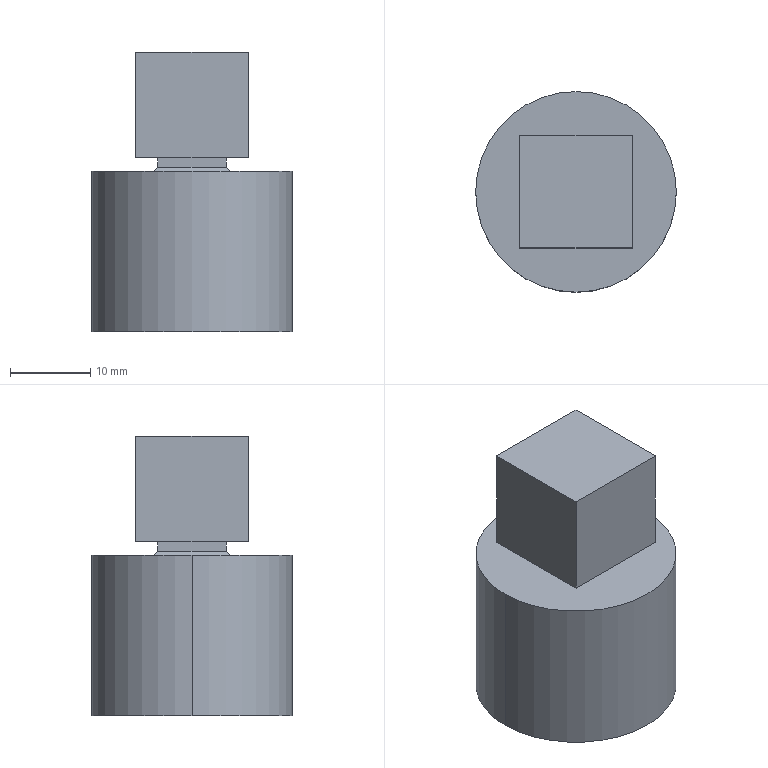Part | SolidWorks | features ICE 3, Chamfer 1, Extrusion 1 | 1 solid | 21 faces | box 25 x 25 x 34.87 mm | volume 7814 mm3 | plane 17 | cylinder 4 | commonest cylinder face diameters 20 x2 25 x2
STEP:
#1=CARTESIAN_POINT('',(10.,0.,15.));
#2=VERTEX_POINT('',#1);
#3=CARTESIAN_POINT('',(-10.,0.,15.));
#4=VERTEX_POINT('',#3);
#5=CARTESIAN_POINT('',(0.,0.,15.));
#6=DIRECTION('',(0.,0.,-1.));
#7=DIRECTION('',(-1.,0.,0.));
#8=AXIS2_PLACEMENT_3D('',#5,#6,#7);
#9=CIRCLE('',#8,10.);
#10=EDGE_CURVE('',#2,#4,#9,.T.);
#11=ORIENTED_EDGE('',*,*,#10,.F.);
#12=CARTESIAN_POINT('',(10.,0.,0.));
#13=VERTEX_POINT('',#12);
#14=CARTESIAN_POINT('',(10.,0.,15.));
#15=DIRECTION('',(0.,0.,-1.));
#16=VECTOR('',#15,1000.);
#17=LINE('',#14,#16);
#18=EDGE_CURVE('',#2,#13,#17,.T.);
#19=ORIENTED_EDGE('',*,*,#18,.T.);
#20=CARTESIAN_POINT('',(-10.,0.,0.));
#21=VERTEX_POINT('',#20);
#22=CARTESIAN_POINT('',(0.,0.,0.));
#23=DIRECTION('',(0.,0.,-1.));
#24=DIRECTION('',(-1.,0.,0.));
#25=AXIS2_PLACEMENT_3D('',#22,#23,#24);
#26=CIRCLE('',#25,10.);
#27=EDGE_CURVE('',#13,#21,#26,.T.);
#28=ORIENTED_EDGE('',*,*,#27,.T.);
#29=CARTESIAN_POINT('',(-10.,0.,15.));
#30=DIRECTION('',(0.,0.,-1.));
#31=VECTOR('',#30,1000.);
#32=LINE('',#29,#31);
#33=EDGE_CURVE('',#4,#21,#32,.T.);
#34=ORIENTED_EDGE('',*,*,#33,.F.);
#35=EDGE_LOOP('',(#11,#19,#28,#34));
#36=FACE_OUTER_BOUND('',#35,.T.);
#37=CARTESIAN_POINT('',(0.,0.,15.));
#38=DIRECTION('',(0.,0.,-1.));
#39=DIRECTION('',(-1.,0.,0.));
#40=AXIS2_PLACEMENT_3D('',#37,#38,#39);
#41=CYLINDRICAL_SURFACE('',#40,10.);
#42=ADVANCED_FACE('',(#36),#41,.F.);
#43=CARTESIAN_POINT('',(12.5,0.,20.));
#44=VERTEX_POINT('',#43);
#45=CARTESIAN_POINT('',(-12.5,0.,20.));
#46=VERTEX_POINT('',#45);
#47=CARTESIAN_POINT('',(0.,0.,20.));
#48=DIRECTION('',(0.,0.,1.));
#49=DIRECTION('',(1.,0.,0.));
#50=AXIS2_PLACEMENT_3D('',#47,#48,#49);
#51=CIRCLE('',#50,12.5);
#52=EDGE_CURVE('',#44,#46,#51,.T.);
#53=ORIENTED_EDGE('',*,*,#52,.F.);
#54=CARTESIAN_POINT('',(12.5,0.,0.));
#55=VERTEX_POINT('',#54);
#56=CARTESIAN_POINT('',(12.5,0.,20.));
#57=DIRECTION('',(0.,0.,-1.));
#58=VECTOR('',#57,1000.);
#59=LINE('',#56,#58);
#60=EDGE_CURVE('',#44,#55,#59,.T.);
#61=ORIENTED_EDGE('',*,*,#60,.T.);
#62=CARTESIAN_POINT('',(-12.5,0.,0.));
#63=VERTEX_POINT('',#62);
#64=CARTESIAN_POINT('',(0.,0.,0.));
#65=DIRECTION('',(0.,0.,1.));
#66=DIRECTION('',(1.,0.,0.));
#67=AXIS2_PLACEMENT_3D('',#64,#65,#66);
#68=CIRCLE('',#67,12.5);
#69=EDGE_CURVE('',#55,#63,#68,.T.);
#70=ORIENTED_EDGE('',*,*,#69,.T.);
#71=CARTESIAN_POINT('',(-12.5,0.,20.));
#72=DIRECTION('',(0.,0.,-1.));
#73=VECTOR('',#72,1000.);
#74=LINE('',#71,#73);
#75=EDGE_CURVE('',#46,#63,#74,.T.);
#76=ORIENTED_EDGE('',*,*,#75,.F.);
#77=EDGE_LOOP('',(#53,#61,#70,#76));
#78=FACE_OUTER_BOUND('',#77,.T.);
#79=CARTESIAN_POINT('',(0.,0.,20.));
#80=DIRECTION('',(0.,0.,-1.));
#81=DIRECTION('',(-1.,0.,0.));
#82=AXIS2_PLACEMENT_3D('',#79,#80,#81);
#83=CYLINDRICAL_SURFACE('',#82,12.5);
#84=ADVANCED_FACE('',(#78),#83,.T.);
#85=ORIENTED_EDGE('',*,*,#60,.F.);
#86=CARTESIAN_POINT('',(0.,0.,20.));
#87=DIRECTION('',(0.,0.,1.));
#88=DIRECTION('',(1.,0.,0.));
#89=AXIS2_PLACEMENT_3D('',#86,#87,#88);
#90=CIRCLE('',#89,12.5);
#91=EDGE_CURVE('',#46,#44,#90,.T.);
#92=ORIENTED_EDGE('',*,*,#91,.F.);
#93=ORIENTED_EDGE('',*,*,#75,.T.);
#94=CARTESIAN_POINT('',(0.,0.,0.));
#95=DIRECTION('',(0.,0.,1.));
#96=DIRECTION('',(1.,0.,0.));
#97=AXIS2_PLACEMENT_3D('',#94,#95,#96);
#98=CIRCLE('',#97,12.5);
#99=EDGE_CURVE('',#63,#55,#98,.T.);
#100=ORIENTED_EDGE('',*,*,#99,.T.);
#101=EDGE_LOOP('',(#85,#92,#93,#100));
#102=FACE_OUTER_BOUND('',#101,.T.);
#103=CARTESIAN_POINT('',(0.,0.,20.));
#104=DIRECTION('',(0.,0.,-1.));
#105=DIRECTION('',(-1.,0.,0.));
#106=AXIS2_PLACEMENT_3D('',#103,#104,#105);
#107=CYLINDRICAL_SURFACE('',#106,12.5);
#108=ADVANCED_FACE('',(#102),#107,.T.);
#109=CARTESIAN_POINT('',(4.75,4.75,20.));
#110=VERTEX_POINT('',#109);
#111=CARTESIAN_POINT('',(4.75,-4.75,20.));
#112=VERTEX_POINT('',#111);
#113=CARTESIAN_POINT('',(4.75,0.,20.));
#114=DIRECTION('',(0.,-1.,0.));
#115=VECTOR('',#114,1000.);
#116=LINE('',#113,#115);
#117=EDGE_CURVE('',#110,#112,#116,.T.);
#118=ORIENTED_EDGE('',*,*,#117,.T.);
#119=CARTESIAN_POINT('',(-4.75,-4.75,20.));
#120=VERTEX_POINT('',#119);
#121=CARTESIAN_POINT('',(0.,-4.75,20.));
#122=DIRECTION('',(-1.,0.,0.));
#123=VECTOR('',#122,1000.);
#124=LINE('',#121,#123);
#125=EDGE_CURVE('',#112,#120,#124,.T.);
#126=ORIENTED_EDGE('',*,*,#125,.T.);
#127=CARTESIAN_POINT('',(-4.75,4.75,20.));
#128=VERTEX_POINT('',#127);
#129=CARTESIAN_POINT('',(-4.75,0.,20.));
#130=DIRECTION('',(0.,1.,0.));
#131=VECTOR('',#130,1000.);
#132=LINE('',#129,#131);
#133=EDGE_CURVE('',#120,#128,#132,.T.);
#134=ORIENTED_EDGE('',*,*,#133,.T.);
#135=CARTESIAN_POINT('',(0.,4.75,20.));
#136=DIRECTION('',(1.,0.,0.));
#137=VECTOR('',#136,1000.);
#138=LINE('',#135,#137);
#139=EDGE_CURVE('',#128,#110,#138,.T.);
#140=ORIENTED_EDGE('',*,*,#139,.T.);
#141=EDGE_LOOP('',(#118,#126,#134,#140));
#142=FACE_BOUND('',#141,.T.);
#143=ORIENTED_EDGE('',*,*,#91,.T.);
#144=ORIENTED_EDGE('',*,*,#52,.T.);
#145=EDGE_LOOP('',(#143,#144));
#146=FACE_OUTER_BOUND('',#145,.T.);
#147=CARTESIAN_POINT('',(0.,0.,20.));
#148=DIRECTION('',(0.,0.,1.));
#149=DIRECTION('',(1.,0.,0.));
#150=AXIS2_PLACEMENT_3D('',#147,#148,#149);
#151=PLANE('',#150);
#152=ADVANCED_FACE('',(#142,#146),#151,.T.);
#153=CARTESIAN_POINT('',(0.,0.,0.));
#154=DIRECTION('',(0.,0.,-1.));
#155=DIRECTION('',(-1.,0.,0.));
#156=AXIS2_PLACEMENT_3D('',#153,#154,#155);
#157=CIRCLE('',#156,10.);
#158=EDGE_CURVE('',#21,#13,#157,.T.);
#159=ORIENTED_EDGE('',*,*,#158,.F.);
#160=ORIENTED_EDGE('',*,*,#27,.F.);
#161=EDGE_LOOP('',(#159,#160));
#162=FACE_BOUND('',#161,.T.);
#163=ORIENTED_EDGE('',*,*,#99,.F.);
#164=ORIENTED_EDGE('',*,*,#69,.F.);
#165=EDGE_LOOP('',(#163,#164));
#166=FACE_OUTER_BOUND('',#165,.T.);
#167=CARTESIAN_POINT('',(0.,0.,0.));
#168=DIRECTION('',(0.,0.,1.));
#169=DIRECTION('',(1.,0.,0.));
#170=AXIS2_PLACEMENT_3D('',#167,#168,#169);
#171=PLANE('',#170);
#172=ADVANCED_FACE('',(#162,#166),#171,.F.);
#173=CARTESIAN_POINT('',(4.25,-4.25,21.7));
#174=VERTEX_POINT('',#173);
#175=CARTESIAN_POINT('',(4.25,-4.25,20.5));
#176=VERTEX_POINT('',#175);
#177=CARTESIAN_POINT('',(4.25,-4.25,21.7));
#178=DIRECTION('',(0.,0.,-1.));
#179=VECTOR('',#178,1000.);
#180=LINE('',#177,#179);
#181=EDGE_CURVE('',#174,#176,#180,.T.);
#182=ORIENTED_EDGE('',*,*,#181,.T.);
#183=CARTESIAN_POINT('',(4.25,4.25,20.5));
#184=VERTEX_POINT('',#183);
#185=CARTESIAN_POINT('',(4.25,-4.25,20.5));
#186=DIRECTION('',(0.,1.,0.));
#187=VECTOR('',#186,1000.);
#188=LINE('',#185,#187);
#189=EDGE_CURVE('',#176,#184,#188,.T.);
#190=ORIENTED_EDGE('',*,*,#189,.T.);
#191=CARTESIAN_POINT('',(4.25,4.25,21.7));
#192=VERTEX_POINT('',#191);
#193=CARTESIAN_POINT('',(4.25,4.25,21.7));
#194=DIRECTION('',(0.,0.,-1.));
#195=VECTOR('',#194,1000.);
#196=LINE('',#193,#195);
#197=EDGE_CURVE('',#192,#184,#196,.T.);
#198=ORIENTED_EDGE('',*,*,#197,.F.);
#199=CARTESIAN_POINT('',(4.25,-4.25,21.7));
#200=DIRECTION('',(0.,1.,0.));
#201=VECTOR('',#200,1000.);
#202=LINE('',#199,#201);
#203=EDGE_CURVE('',#174,#192,#202,.T.);
#204=ORIENTED_EDGE('',*,*,#203,.F.);
#205=EDGE_LOOP('',(#182,#190,#198,#204));
#206=FACE_OUTER_BOUND('',#205,.T.);
#207=CARTESIAN_POINT('',(4.25,-4.25,21.7));
#208=DIRECTION('',(-1.,0.,0.));
#209=DIRECTION('',(0.,0.,1.));
#210=AXIS2_PLACEMENT_3D('',#207,#208,#209);
#211=PLANE('',#210);
#212=ADVANCED_FACE('',(#206),#211,.F.);
#213=ORIENTED_EDGE('',*,*,#197,.T.);
#214=CARTESIAN_POINT('',(-4.25,4.25,20.5));
#215=VERTEX_POINT('',#214);
#216=CARTESIAN_POINT('',(-4.25,4.25,20.5));
#217=DIRECTION('',(-1.,0.,0.));
#218=VECTOR('',#217,1000.);
#219=LINE('',#216,#218);
#220=EDGE_CURVE('',#184,#215,#219,.T.);
#221=ORIENTED_EDGE('',*,*,#220,.T.);
#222=CARTESIAN_POINT('',(-4.25,4.25,21.7));
#223=VERTEX_POINT('',#222);
#224=CARTESIAN_POINT('',(-4.25,4.25,21.7));
#225=DIRECTION('',(0.,0.,-1.));
#226=VECTOR('',#225,1000.);
#227=LINE('',#224,#226);
#228=EDGE_CURVE('',#223,#215,#227,.T.);
#229=ORIENTED_EDGE('',*,*,#228,.F.);
#230=CARTESIAN_POINT('',(-4.25,4.25,21.7));
#231=DIRECTION('',(-1.,0.,0.));
#232=VECTOR('',#231,1000.);
#233=LINE('',#230,#232);
#234=EDGE_CURVE('',#192,#223,#233,.T.);
#235=ORIENTED_EDGE('',*,*,#234,.F.);
#236=EDGE_LOOP('',(#213,#221,#229,#235));
#237=FACE_OUTER_BOUND('',#236,.T.);
#238=CARTESIAN_POINT('',(-4.25,4.25,21.7));
#239=DIRECTION('',(0.,-1.,0.));
#240=DIRECTION('',(0.,0.,-1.));
#241=AXIS2_PLACEMENT_3D('',#238,#239,#240);
#242=PLANE('',#241);
#243=ADVANCED_FACE('',(#237),#242,.F.);
#244=ORIENTED_EDGE('',*,*,#228,.T.);
#245=CARTESIAN_POINT('',(-4.25,-4.25,20.5));
#246=VERTEX_POINT('',#245);
#247=CARTESIAN_POINT('',(-4.25,-4.25,20.5));
#248=DIRECTION('',(0.,-1.,0.));
#249=VECTOR('',#248,1000.);
#250=LINE('',#247,#249);
#251=EDGE_CURVE('',#215,#246,#250,.T.);
#252=ORIENTED_EDGE('',*,*,#251,.T.);
#253=CARTESIAN_POINT('',(-4.25,-4.25,21.7));
#254=VERTEX_POINT('',#253);
#255=CARTESIAN_POINT('',(-4.25,-4.25,21.7));
#256=DIRECTION('',(0.,0.,-1.));
#257=VECTOR('',#256,1000.);
#258=LINE('',#255,#257);
#259=EDGE_CURVE('',#254,#246,#258,.T.);
#260=ORIENTED_EDGE('',*,*,#259,.F.);
#261=CARTESIAN_POINT('',(-4.25,-4.25,21.7));
#262=DIRECTION('',(0.,-1.,0.));
#263=VECTOR('',#262,1000.);
#264=LINE('',#261,#263);
#265=EDGE_CURVE('',#223,#254,#264,.T.);
#266=ORIENTED_EDGE('',*,*,#265,.F.);
#267=EDGE_LOOP('',(#244,#252,#260,#266));
#268=FACE_OUTER_BOUND('',#267,.T.);
#269=CARTESIAN_POINT('',(-4.25,-4.25,21.7));
#270=DIRECTION('',(1.,0.,0.));
#271=DIRECTION('',(0.,0.,-1.));
#272=AXIS2_PLACEMENT_3D('',#269,#270,#271);
#273=PLANE('',#272);
#274=ADVANCED_FACE('',(#268),#273,.F.);
#275=ORIENTED_EDGE('',*,*,#259,.T.);
#276=CARTESIAN_POINT('',(-4.25,-4.25,20.5));
#277=DIRECTION('',(1.,0.,0.));
#278=VECTOR('',#277,1000.);
#279=LINE('',#276,#278);
#280=EDGE_CURVE('',#246,#176,#279,.T.);
#281=ORIENTED_EDGE('',*,*,#280,.T.);
#282=ORIENTED_EDGE('',*,*,#181,.F.);
#283=CARTESIAN_POINT('',(-4.25,-4.25,21.7));
#284=DIRECTION('',(1.,0.,0.));
#285=VECTOR('',#284,1000.);
#286=LINE('',#283,#285);
#287=EDGE_CURVE('',#254,#174,#286,.T.);
#288=ORIENTED_EDGE('',*,*,#287,.F.);
#289=EDGE_LOOP('',(#275,#281,#282,#288));
#290=FACE_OUTER_BOUND('',#289,.T.);
#291=CARTESIAN_POINT('',(-4.25,-4.25,21.7));
#292=DIRECTION('',(0.,1.,0.));
#293=DIRECTION('',(0.,0.,1.));
#294=AXIS2_PLACEMENT_3D('',#291,#292,#293);
#295=PLANE('',#294);
#296=ADVANCED_FACE('',(#290),#295,.F.);
#297=CARTESIAN_POINT('',(7.,-7.,21.7));
#298=VERTEX_POINT('',#297);
#299=CARTESIAN_POINT('',(7.,7.,21.7));
#300=VERTEX_POINT('',#299);
#301=CARTESIAN_POINT('',(7.,-7.,21.7));
#302=DIRECTION('',(0.,1.,0.));
#303=VECTOR('',#302,1000.);
#304=LINE('',#301,#303);
#305=EDGE_CURVE('',#298,#300,#304,.T.);
#306=ORIENTED_EDGE('',*,*,#305,.T.);
#307=CARTESIAN_POINT('',(7.,7.,34.87));
#308=VERTEX_POINT('',#307);
#309=CARTESIAN_POINT('',(7.,7.,34.87));
#310=DIRECTION('',(0.,0.,-1.));
#311=VECTOR('',#310,1000.);
#312=LINE('',#309,#311);
#313=EDGE_CURVE('',#308,#300,#312,.T.);
#314=ORIENTED_EDGE('',*,*,#313,.F.);
#315=CARTESIAN_POINT('',(7.,-7.,34.87));
#316=VERTEX_POINT('',#315);
#317=CARTESIAN_POINT('',(7.,-7.,34.87));
#318=DIRECTION('',(0.,1.,0.));
#319=VECTOR('',#318,1000.);
#320=LINE('',#317,#319);
#321=EDGE_CURVE('',#316,#308,#320,.T.);
#322=ORIENTED_EDGE('',*,*,#321,.F.);
#323=CARTESIAN_POINT('',(7.,-7.,34.87));
#324=DIRECTION('',(0.,0.,-1.));
#325=VECTOR('',#324,1000.);
#326=LINE('',#323,#325);
#327=EDGE_CURVE('',#316,#298,#326,.T.);
#328=ORIENTED_EDGE('',*,*,#327,.T.);
#329=EDGE_LOOP('',(#306,#314,#322,#328));
#330=FACE_OUTER_BOUND('',#329,.T.);
#331=CARTESIAN_POINT('',(7.,-7.,34.87));
#332=DIRECTION('',(-1.,0.,0.));
#333=DIRECTION('',(0.,0.,1.));
#334=AXIS2_PLACEMENT_3D('',#331,#332,#333);
#335=PLANE('',#334);
#336=ADVANCED_FACE('',(#330),#335,.F.);
#337=CARTESIAN_POINT('',(-7.,7.,21.7));
#338=VERTEX_POINT('',#337);
#339=CARTESIAN_POINT('',(-7.,7.,21.7));
#340=DIRECTION('',(-1.,0.,0.));
#341=VECTOR('',#340,1000.);
#342=LINE('',#339,#341);
#343=EDGE_CURVE('',#300,#338,#342,.T.);
#344=ORIENTED_EDGE('',*,*,#343,.T.);
#345=CARTESIAN_POINT('',(-7.,7.,34.87));
#346=VERTEX_POINT('',#345);
#347=CARTESIAN_POINT('',(-7.,7.,34.87));
#348=DIRECTION('',(0.,0.,-1.));
#349=VECTOR('',#348,1000.);
#350=LINE('',#347,#349);
#351=EDGE_CURVE('',#346,#338,#350,.T.);
#352=ORIENTED_EDGE('',*,*,#351,.F.);
#353=CARTESIAN_POINT('',(-7.,7.,34.87));
#354=DIRECTION('',(-1.,0.,0.));
#355=VECTOR('',#354,1000.);
#356=LINE('',#353,#355);
#357=EDGE_CURVE('',#308,#346,#356,.T.);
#358=ORIENTED_EDGE('',*,*,#357,.F.);
#359=ORIENTED_EDGE('',*,*,#313,.T.);
#360=EDGE_LOOP('',(#344,#352,#358,#359));
#361=FACE_OUTER_BOUND('',#360,.T.);
#362=CARTESIAN_POINT('',(-7.,7.,34.87));
#363=DIRECTION('',(0.,-1.,0.));
#364=DIRECTION('',(0.,0.,-1.));
#365=AXIS2_PLACEMENT_3D('',#362,#363,#364);
#366=PLANE('',#365);
#367=ADVANCED_FACE('',(#361),#366,.F.);
#368=CARTESIAN_POINT('',(-7.,-7.,21.7));
#369=VERTEX_POINT('',#368);
#370=CARTESIAN_POINT('',(-7.,-7.,21.7));
#371=DIRECTION('',(0.,-1.,0.));
#372=VECTOR('',#371,1000.);
#373=LINE('',#370,#372);
#374=EDGE_CURVE('',#338,#369,#373,.T.);
#375=ORIENTED_EDGE('',*,*,#374,.T.);
#376=CARTESIAN_POINT('',(-7.,-7.,34.87));
#377=VERTEX_POINT('',#376);
#378=CARTESIAN_POINT('',(-7.,-7.,34.87));
#379=DIRECTION('',(0.,0.,-1.));
#380=VECTOR('',#379,1000.);
#381=LINE('',#378,#380);
#382=EDGE_CURVE('',#377,#369,#381,.T.);
#383=ORIENTED_EDGE('',*,*,#382,.F.);
#384=CARTESIAN_POINT('',(-7.,-7.,34.87));
#385=DIRECTION('',(0.,-1.,0.));
#386=VECTOR('',#385,1000.);
#387=LINE('',#384,#386);
#388=EDGE_CURVE('',#346,#377,#387,.T.);
#389=ORIENTED_EDGE('',*,*,#388,.F.);
#390=ORIENTED_EDGE('',*,*,#351,.T.);
#391=EDGE_LOOP('',(#375,#383,#389,#390));
#392=FACE_OUTER_BOUND('',#391,.T.);
#393=CARTESIAN_POINT('',(-7.,-7.,34.87));
#394=DIRECTION('',(1.,0.,0.));
#395=DIRECTION('',(0.,0.,-1.));
#396=AXIS2_PLACEMENT_3D('',#393,#394,#395);
#397=PLANE('',#396);
#398=ADVANCED_FACE('',(#392),#397,.F.);
#399=CARTESIAN_POINT('',(-7.,-7.,21.7));
#400=DIRECTION('',(1.,0.,0.));
#401=VECTOR('',#400,1000.);
#402=LINE('',#399,#401);
#403=EDGE_CURVE('',#369,#298,#402,.T.);
#404=ORIENTED_EDGE('',*,*,#403,.T.);
#405=ORIENTED_EDGE('',*,*,#327,.F.);
#406=CARTESIAN_POINT('',(-7.,-7.,34.87));
#407=DIRECTION('',(1.,0.,0.));
#408=VECTOR('',#407,1000.);
#409=LINE('',#406,#408);
#410=EDGE_CURVE('',#377,#316,#409,.T.);
#411=ORIENTED_EDGE('',*,*,#410,.F.);
#412=ORIENTED_EDGE('',*,*,#382,.T.);
#413=EDGE_LOOP('',(#404,#405,#411,#412));
#414=FACE_OUTER_BOUND('',#413,.T.);
#415=CARTESIAN_POINT('',(-7.,-7.,34.87));
#416=DIRECTION('',(0.,1.,0.));
#417=DIRECTION('',(0.,0.,1.));
#418=AXIS2_PLACEMENT_3D('',#415,#416,#417);
#419=PLANE('',#418);
#420=ADVANCED_FACE('',(#414),#419,.F.);
#421=ORIENTED_EDGE('',*,*,#321,.T.);
#422=ORIENTED_EDGE('',*,*,#357,.T.);
#423=ORIENTED_EDGE('',*,*,#388,.T.);
#424=ORIENTED_EDGE('',*,*,#410,.T.);
#425=EDGE_LOOP('',(#421,#422,#423,#424));
#426=FACE_OUTER_BOUND('',#425,.T.);
#427=CARTESIAN_POINT('',(0.,0.,34.87));
#428=DIRECTION('',(0.,0.,-1.));
#429=DIRECTION('',(-1.,0.,0.));
#430=AXIS2_PLACEMENT_3D('',#427,#428,#429);
#431=PLANE('',#430);
#432=ADVANCED_FACE('',(#426),#431,.F.);
#433=ORIENTED_EDGE('',*,*,#287,.T.);
#434=ORIENTED_EDGE('',*,*,#203,.T.);
#435=ORIENTED_EDGE('',*,*,#234,.T.);
#436=ORIENTED_EDGE('',*,*,#265,.T.);
#437=EDGE_LOOP('',(#433,#434,#435,#436));
#438=FACE_BOUND('',#437,.T.);
#439=ORIENTED_EDGE('',*,*,#305,.F.);
#440=ORIENTED_EDGE('',*,*,#403,.F.);
#441=ORIENTED_EDGE('',*,*,#374,.F.);
#442=ORIENTED_EDGE('',*,*,#343,.F.);
#443=EDGE_LOOP('',(#439,#440,#441,#442));
#444=FACE_OUTER_BOUND('',#443,.T.);
#445=CARTESIAN_POINT('',(0.,0.,21.7));
#446=DIRECTION('',(0.,0.,-1.));
#447=DIRECTION('',(-1.,0.,0.));
#448=AXIS2_PLACEMENT_3D('',#445,#446,#447);
#449=PLANE('',#448);
#450=ADVANCED_FACE('',(#438,#444),#449,.T.);
#451=ORIENTED_EDGE('',*,*,#18,.F.);
#452=CARTESIAN_POINT('',(0.,0.,15.));
#453=DIRECTION('',(0.,0.,-1.));
#454=DIRECTION('',(-1.,0.,0.));
#455=AXIS2_PLACEMENT_3D('',#452,#453,#454);
#456=CIRCLE('',#455,10.);
#457=EDGE_CURVE('',#4,#2,#456,.T.);
#458=ORIENTED_EDGE('',*,*,#457,.F.);
#459=ORIENTED_EDGE('',*,*,#33,.T.);
#460=ORIENTED_EDGE('',*,*,#158,.T.);
#461=EDGE_LOOP('',(#451,#458,#459,#460));
#462=FACE_OUTER_BOUND('',#461,.T.);
#463=CARTESIAN_POINT('',(0.,0.,15.));
#464=DIRECTION('',(0.,0.,-1.));
#465=DIRECTION('',(-1.,0.,0.));
#466=AXIS2_PLACEMENT_3D('',#463,#464,#465);
#467=CYLINDRICAL_SURFACE('',#466,10.);
#468=ADVANCED_FACE('',(#462),#467,.F.);
#469=ORIENTED_EDGE('',*,*,#457,.T.);
#470=ORIENTED_EDGE('',*,*,#10,.T.);
#471=EDGE_LOOP('',(#469,#470));
#472=FACE_OUTER_BOUND('',#471,.T.);
#473=CARTESIAN_POINT('',(0.,0.,15.));
#474=DIRECTION('',(0.,0.,-1.));
#475=DIRECTION('',(-1.,0.,0.));
#476=AXIS2_PLACEMENT_3D('',#473,#474,#475);
#477=PLANE('',#476);
#478=ADVANCED_FACE('',(#472),#477,.T.);
#479=CARTESIAN_POINT('',(1.417,1.417,23.333));
#480=DIRECTION('',(-0.5774,-0.5774,0.5774));
#481=VECTOR('',#480,1000.);
#482=LINE('',#479,#481);
#483=EDGE_CURVE('',#110,#184,#482,.T.);
#484=ORIENTED_EDGE('',*,*,#483,.F.);
#485=ORIENTED_EDGE('',*,*,#139,.F.);
#486=CARTESIAN_POINT('',(-4.25,4.25,20.5));
#487=DIRECTION('',(-0.5774,0.5774,-0.5774));
#488=VECTOR('',#487,1000.);
#489=LINE('',#486,#488);
#490=EDGE_CURVE('',#215,#128,#489,.T.);
#491=ORIENTED_EDGE('',*,*,#490,.F.);
#492=ORIENTED_EDGE('',*,*,#220,.F.);
#493=EDGE_LOOP('',(#484,#485,#491,#492));
#494=FACE_OUTER_BOUND('',#493,.T.);
#495=CARTESIAN_POINT('',(-4.25,4.25,20.5));
#496=DIRECTION('',(0.,-0.7071,-0.7071));
#497=DIRECTION('',(-1.,0.,0.));
#498=AXIS2_PLACEMENT_3D('',#495,#496,#497);
#499=PLANE('',#498);
#500=ADVANCED_FACE('',(#494),#499,.F.);
#501=ORIENTED_EDGE('',*,*,#490,.T.);
#502=ORIENTED_EDGE('',*,*,#133,.F.);
#503=CARTESIAN_POINT('',(-4.25,-4.25,20.5));
#504=DIRECTION('',(-0.5774,-0.5774,-0.5774));
#505=VECTOR('',#504,1000.);
#506=LINE('',#503,#505);
#507=EDGE_CURVE('',#246,#120,#506,.T.);
#508=ORIENTED_EDGE('',*,*,#507,.F.);
#509=ORIENTED_EDGE('',*,*,#251,.F.);
#510=EDGE_LOOP('',(#501,#502,#508,#509));
#511=FACE_OUTER_BOUND('',#510,.T.);
#512=CARTESIAN_POINT('',(-4.25,-4.25,20.5));
#513=DIRECTION('',(0.7071,0.,-0.7071));
#514=DIRECTION('',(0.,-1.,0.));
#515=AXIS2_PLACEMENT_3D('',#512,#513,#514);
#516=PLANE('',#515);
#517=ADVANCED_FACE('',(#511),#516,.F.);
#518=ORIENTED_EDGE('',*,*,#483,.T.);
#519=ORIENTED_EDGE('',*,*,#189,.F.);
#520=CARTESIAN_POINT('',(4.25,-4.25,20.5));
#521=DIRECTION('',(-0.5774,0.5774,0.5774));
#522=VECTOR('',#521,1000.);
#523=LINE('',#520,#522);
#524=EDGE_CURVE('',#112,#176,#523,.T.);
#525=ORIENTED_EDGE('',*,*,#524,.F.);
#526=ORIENTED_EDGE('',*,*,#117,.F.);
#527=EDGE_LOOP('',(#518,#519,#525,#526));
#528=FACE_OUTER_BOUND('',#527,.T.);
#529=CARTESIAN_POINT('',(4.25,-4.25,20.5));
#530=DIRECTION('',(-0.7071,0.,-0.7071));
#531=DIRECTION('',(0.,1.,0.));
#532=AXIS2_PLACEMENT_3D('',#529,#530,#531);
#533=PLANE('',#532);
#534=ADVANCED_FACE('',(#528),#533,.F.);
#535=ORIENTED_EDGE('',*,*,#507,.T.);
#536=ORIENTED_EDGE('',*,*,#125,.F.);
#537=ORIENTED_EDGE('',*,*,#524,.T.);
#538=ORIENTED_EDGE('',*,*,#280,.F.);
#539=EDGE_LOOP('',(#535,#536,#537,#538));
#540=FACE_OUTER_BOUND('',#539,.T.);
#541=CARTESIAN_POINT('',(-4.25,-4.25,20.5));
#542=DIRECTION('',(0.,0.7071,-0.7071));
#543=DIRECTION('',(1.,0.,0.));
#544=AXIS2_PLACEMENT_3D('',#541,#542,#543);
#545=PLANE('',#544);
#546=ADVANCED_FACE('',(#540),#545,.F.);
#547=CLOSED_SHELL('',(#42,#84,#108,#152,#172,#212,#243,#274,#296,#336,#367,#398,#420,#432,#450,#468,#478,#500,#517,#534,#546));
#548=MANIFOLD_SOLID_BREP('',#547);
#549=CARTESIAN_POINT('',(0.,0.,0.));
#550=DIRECTION('',(0.,0.,1.));
#551=DIRECTION('',(1.,0.,0.));
#552=AXIS2_PLACEMENT_3D('',#549,#550,#551);
#553=(LENGTH_UNIT()NAMED_UNIT(*)SI_UNIT(.MILLI.,.METRE.));
#554=UNCERTAINTY_MEASURE_WITH_UNIT(LENGTH_MEASURE(0.00001),#553,'','');
#555=(NAMED_UNIT(*)PLANE_ANGLE_UNIT()SI_UNIT($,.RADIAN.));
#556=(NAMED_UNIT(*)SI_UNIT($,.STERADIAN.)SOLID_ANGLE_UNIT());
#557=(GEOMETRIC_REPRESENTATION_CONTEXT(3)GLOBAL_UNCERTAINTY_ASSIGNED_CONTEXT((#554))GLOBAL_UNIT_ASSIGNED_CONTEXT((#553,#555,#556))REPRESENTATION_CONTEXT('',''));
#558=ADVANCED_BREP_SHAPE_REPRESENTATION('',(#548,#552),#557);